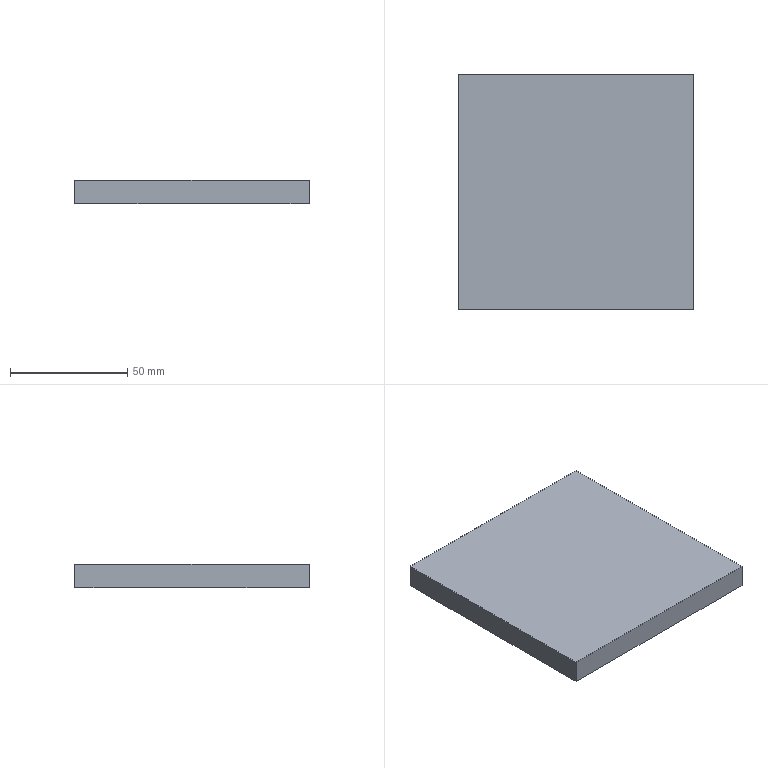Part | NX | features solid 2 | 1 solid | 13 faces | box 100 x 100 x 10 mm | volume 100000 mm3 | plane 13
STEP:
#1=CARTESIAN_POINT('',(490.,-590.,-30.));
#2=VERTEX_POINT('',#1);
#3=CARTESIAN_POINT('',(480.,-590.,-30.));
#4=VERTEX_POINT('',#3);
#5=CARTESIAN_POINT('',(490.,-590.,-30.));
#6=DIRECTION('',(-1.,0.,0.));
#7=VECTOR('',#6,1000.);
#8=LINE('',#5,#7);
#9=EDGE_CURVE('',#2,#4,#8,.T.);
#10=ORIENTED_EDGE('',*,*,#9,.T.);
#11=CARTESIAN_POINT('',(490.,-580.,-30.));
#12=VERTEX_POINT('',#11);
#13=CARTESIAN_POINT('',(430.,-640.,-30.));
#14=DIRECTION('',(0.7071,0.7071,0.));
#15=VECTOR('',#14,1000.);
#16=LINE('',#13,#15);
#17=EDGE_CURVE('',#4,#12,#16,.T.);
#18=ORIENTED_EDGE('',*,*,#17,.T.);
#19=CARTESIAN_POINT('',(490.,-490.,-30.));
#20=DIRECTION('',(0.,-1.,0.));
#21=VECTOR('',#20,1000.);
#22=LINE('',#19,#21);
#23=EDGE_CURVE('',#12,#2,#22,.T.);
#24=ORIENTED_EDGE('',*,*,#23,.T.);
#25=EDGE_LOOP('',(#10,#18,#24));
#26=FACE_BOUND('',#25,.T.);
#27=CARTESIAN_POINT('',(500.,-490.,-30.));
#28=DIRECTION('',(0.,0.,-1.));
#29=DIRECTION('',(0.,-1.,0.));
#30=AXIS2_PLACEMENT_3D('',#27,#28,#29);
#31=PLANE('',#30);
#32=ADVANCED_FACE('',(#26),#31,.T.);
#33=ORIENTED_EDGE('',*,*,#17,.F.);
#34=CARTESIAN_POINT('',(450.,-590.,-30.));
#35=VERTEX_POINT('',#34);
#36=CARTESIAN_POINT('',(490.,-590.,-30.));
#37=DIRECTION('',(-1.,0.,0.));
#38=VECTOR('',#37,1000.);
#39=LINE('',#36,#38);
#40=EDGE_CURVE('',#4,#35,#39,.T.);
#41=ORIENTED_EDGE('',*,*,#40,.T.);
#42=CARTESIAN_POINT('',(490.,-550.,-30.));
#43=VERTEX_POINT('',#42);
#44=CARTESIAN_POINT('',(400.,-640.,-30.));
#45=DIRECTION('',(0.7071,0.7071,0.));
#46=VECTOR('',#45,1000.);
#47=LINE('',#44,#46);
#48=EDGE_CURVE('',#35,#43,#47,.T.);
#49=ORIENTED_EDGE('',*,*,#48,.T.);
#50=CARTESIAN_POINT('',(490.,-490.,-30.));
#51=DIRECTION('',(0.,-1.,0.));
#52=VECTOR('',#51,1000.);
#53=LINE('',#50,#52);
#54=EDGE_CURVE('',#43,#12,#53,.T.);
#55=ORIENTED_EDGE('',*,*,#54,.T.);
#56=EDGE_LOOP('',(#33,#41,#49,#55));
#57=FACE_BOUND('',#56,.T.);
#58=CARTESIAN_POINT('',(500.,-490.,-30.));
#59=DIRECTION('',(0.,0.,-1.));
#60=DIRECTION('',(0.,-1.,0.));
#61=AXIS2_PLACEMENT_3D('',#58,#59,#60);
#62=PLANE('',#61);
#63=ADVANCED_FACE('',(#57),#62,.T.);
#64=ORIENTED_EDGE('',*,*,#48,.F.);
#65=CARTESIAN_POINT('',(420.,-590.,-30.));
#66=VERTEX_POINT('',#65);
#67=CARTESIAN_POINT('',(490.,-590.,-30.));
#68=DIRECTION('',(-1.,0.,0.));
#69=VECTOR('',#68,1000.);
#70=LINE('',#67,#69);
#71=EDGE_CURVE('',#35,#66,#70,.T.);
#72=ORIENTED_EDGE('',*,*,#71,.T.);
#73=CARTESIAN_POINT('',(490.,-520.,-30.));
#74=VERTEX_POINT('',#73);
#75=CARTESIAN_POINT('',(370.,-640.,-30.));
#76=DIRECTION('',(0.7071,0.7071,0.));
#77=VECTOR('',#76,1000.);
#78=LINE('',#75,#77);
#79=EDGE_CURVE('',#66,#74,#78,.T.);
#80=ORIENTED_EDGE('',*,*,#79,.T.);
#81=CARTESIAN_POINT('',(490.,-490.,-30.));
#82=DIRECTION('',(0.,-1.,0.));
#83=VECTOR('',#82,1000.);
#84=LINE('',#81,#83);
#85=EDGE_CURVE('',#74,#43,#84,.T.);
#86=ORIENTED_EDGE('',*,*,#85,.T.);
#87=EDGE_LOOP('',(#64,#72,#80,#86));
#88=FACE_BOUND('',#87,.T.);
#89=CARTESIAN_POINT('',(500.,-490.,-30.));
#90=DIRECTION('',(0.,0.,-1.));
#91=DIRECTION('',(0.,-1.,0.));
#92=AXIS2_PLACEMENT_3D('',#89,#90,#91);
#93=PLANE('',#92);
#94=ADVANCED_FACE('',(#88),#93,.T.);
#95=ORIENTED_EDGE('',*,*,#79,.F.);
#96=CARTESIAN_POINT('',(390.,-590.,-30.));
#97=VERTEX_POINT('',#96);
#98=CARTESIAN_POINT('',(490.,-590.,-30.));
#99=DIRECTION('',(-1.,0.,0.));
#100=VECTOR('',#99,1000.);
#101=LINE('',#98,#100);
#102=EDGE_CURVE('',#66,#97,#101,.T.);
#103=ORIENTED_EDGE('',*,*,#102,.T.);
#104=CARTESIAN_POINT('',(490.,-490.,-30.));
#105=VERTEX_POINT('',#104);
#106=CARTESIAN_POINT('',(340.,-640.,-30.));
#107=DIRECTION('',(0.7071,0.7071,0.));
#108=VECTOR('',#107,1000.);
#109=LINE('',#106,#108);
#110=EDGE_CURVE('',#97,#105,#109,.T.);
#111=ORIENTED_EDGE('',*,*,#110,.T.);
#112=CARTESIAN_POINT('',(490.,-490.,-30.));
#113=DIRECTION('',(0.,-1.,0.));
#114=VECTOR('',#113,1000.);
#115=LINE('',#112,#114);
#116=EDGE_CURVE('',#105,#74,#115,.T.);
#117=ORIENTED_EDGE('',*,*,#116,.T.);
#118=EDGE_LOOP('',(#95,#103,#111,#117));
#119=FACE_BOUND('',#118,.T.);
#120=CARTESIAN_POINT('',(500.,-490.,-30.));
#121=DIRECTION('',(0.,0.,-1.));
#122=DIRECTION('',(0.,-1.,0.));
#123=AXIS2_PLACEMENT_3D('',#120,#121,#122);
#124=PLANE('',#123);
#125=ADVANCED_FACE('',(#119),#124,.T.);
#126=CARTESIAN_POINT('',(390.,-560.,-30.));
#127=VERTEX_POINT('',#126);
#128=CARTESIAN_POINT('',(390.,-490.,-30.));
#129=DIRECTION('',(0.,-1.,0.));
#130=VECTOR('',#129,1000.);
#131=LINE('',#128,#130);
#132=EDGE_CURVE('',#97,#127,#131,.F.);
#133=ORIENTED_EDGE('',*,*,#132,.T.);
#134=CARTESIAN_POINT('',(460.,-490.,-30.));
#135=VERTEX_POINT('',#134);
#136=CARTESIAN_POINT('',(310.,-640.,-30.));
#137=DIRECTION('',(0.7071,0.7071,0.));
#138=VECTOR('',#137,1000.);
#139=LINE('',#136,#138);
#140=EDGE_CURVE('',#127,#135,#139,.T.);
#141=ORIENTED_EDGE('',*,*,#140,.T.);
#142=CARTESIAN_POINT('',(500.,-490.,-30.));
#143=DIRECTION('',(1.,0.,0.));
#144=VECTOR('',#143,1000.);
#145=LINE('',#142,#144);
#146=EDGE_CURVE('',#105,#135,#145,.F.);
#147=ORIENTED_EDGE('',*,*,#146,.F.);
#148=ORIENTED_EDGE('',*,*,#110,.F.);
#149=EDGE_LOOP('',(#133,#141,#147,#148));
#150=FACE_BOUND('',#149,.T.);
#151=CARTESIAN_POINT('',(500.,-490.,-30.));
#152=DIRECTION('',(0.,0.,-1.));
#153=DIRECTION('',(0.,-1.,0.));
#154=AXIS2_PLACEMENT_3D('',#151,#152,#153);
#155=PLANE('',#154);
#156=ADVANCED_FACE('',(#150),#155,.T.);
#157=CARTESIAN_POINT('',(390.,-530.,-30.));
#158=VERTEX_POINT('',#157);
#159=CARTESIAN_POINT('',(390.,-590.,-30.));
#160=DIRECTION('',(0.,1.,0.));
#161=VECTOR('',#160,1000.);
#162=LINE('',#159,#161);
#163=EDGE_CURVE('',#158,#127,#162,.F.);
#164=ORIENTED_EDGE('',*,*,#163,.F.);
#165=CARTESIAN_POINT('',(430.,-490.,-30.));
#166=VERTEX_POINT('',#165);
#167=CARTESIAN_POINT('',(280.,-640.,-30.));
#168=DIRECTION('',(0.7071,0.7071,0.));
#169=VECTOR('',#168,1000.);
#170=LINE('',#167,#169);
#171=EDGE_CURVE('',#158,#166,#170,.T.);
#172=ORIENTED_EDGE('',*,*,#171,.T.);
#173=CARTESIAN_POINT('',(500.,-490.,-30.));
#174=DIRECTION('',(1.,0.,0.));
#175=VECTOR('',#174,1000.);
#176=LINE('',#173,#175);
#177=EDGE_CURVE('',#135,#166,#176,.F.);
#178=ORIENTED_EDGE('',*,*,#177,.F.);
#179=ORIENTED_EDGE('',*,*,#140,.F.);
#180=EDGE_LOOP('',(#164,#172,#178,#179));
#181=FACE_BOUND('',#180,.T.);
#182=CARTESIAN_POINT('',(500.,-490.,-30.));
#183=DIRECTION('',(0.,0.,-1.));
#184=DIRECTION('',(0.,-1.,0.));
#185=AXIS2_PLACEMENT_3D('',#182,#183,#184);
#186=PLANE('',#185);
#187=ADVANCED_FACE('',(#181),#186,.T.);
#188=CARTESIAN_POINT('',(390.,-490.,-30.));
#189=VERTEX_POINT('',#188);
#190=CARTESIAN_POINT('',(390.,-500.,-30.));
#191=VERTEX_POINT('',#190);
#192=CARTESIAN_POINT('',(390.,-590.,-30.));
#193=DIRECTION('',(0.,1.,0.));
#194=VECTOR('',#193,1000.);
#195=LINE('',#192,#194);
#196=EDGE_CURVE('',#189,#191,#195,.F.);
#197=ORIENTED_EDGE('',*,*,#196,.F.);
#198=CARTESIAN_POINT('',(400.,-490.,-30.));
#199=VERTEX_POINT('',#198);
#200=CARTESIAN_POINT('',(500.,-490.,-30.));
#201=DIRECTION('',(1.,0.,0.));
#202=VECTOR('',#201,1000.);
#203=LINE('',#200,#202);
#204=EDGE_CURVE('',#199,#189,#203,.F.);
#205=ORIENTED_EDGE('',*,*,#204,.F.);
#206=CARTESIAN_POINT('',(250.,-640.,-30.));
#207=DIRECTION('',(0.7071,0.7071,0.));
#208=VECTOR('',#207,1000.);
#209=LINE('',#206,#208);
#210=EDGE_CURVE('',#191,#199,#209,.T.);
#211=ORIENTED_EDGE('',*,*,#210,.F.);
#212=EDGE_LOOP('',(#197,#205,#211));
#213=FACE_BOUND('',#212,.T.);
#214=CARTESIAN_POINT('',(500.,-490.,-30.));
#215=DIRECTION('',(0.,0.,-1.));
#216=DIRECTION('',(0.,-1.,0.));
#217=AXIS2_PLACEMENT_3D('',#214,#215,#216);
#218=PLANE('',#217);
#219=ADVANCED_FACE('',(#213),#218,.T.);
#220=ORIENTED_EDGE('',*,*,#171,.F.);
#221=CARTESIAN_POINT('',(390.,-590.,-30.));
#222=DIRECTION('',(0.,1.,0.));
#223=VECTOR('',#222,1000.);
#224=LINE('',#221,#223);
#225=EDGE_CURVE('',#191,#158,#224,.F.);
#226=ORIENTED_EDGE('',*,*,#225,.F.);
#227=ORIENTED_EDGE('',*,*,#210,.T.);
#228=CARTESIAN_POINT('',(500.,-490.,-30.));
#229=DIRECTION('',(1.,0.,0.));
#230=VECTOR('',#229,1000.);
#231=LINE('',#228,#230);
#232=EDGE_CURVE('',#166,#199,#231,.F.);
#233=ORIENTED_EDGE('',*,*,#232,.F.);
#234=EDGE_LOOP('',(#220,#226,#227,#233));
#235=FACE_BOUND('',#234,.T.);
#236=CARTESIAN_POINT('',(500.,-490.,-30.));
#237=DIRECTION('',(0.,0.,-1.));
#238=DIRECTION('',(0.,-1.,0.));
#239=AXIS2_PLACEMENT_3D('',#236,#237,#238);
#240=PLANE('',#239);
#241=ADVANCED_FACE('',(#235),#240,.T.);
#242=ORIENTED_EDGE('',*,*,#146,.T.);
#243=ORIENTED_EDGE('',*,*,#177,.T.);
#244=ORIENTED_EDGE('',*,*,#232,.T.);
#245=ORIENTED_EDGE('',*,*,#204,.T.);
#246=CARTESIAN_POINT('',(390.,-490.,-20.));
#247=VERTEX_POINT('',#246);
#248=CARTESIAN_POINT('',(390.,-490.,-30.));
#249=DIRECTION('',(0.,0.,1.));
#250=VECTOR('',#249,1000.);
#251=LINE('',#248,#250);
#252=EDGE_CURVE('',#189,#247,#251,.T.);
#253=ORIENTED_EDGE('',*,*,#252,.T.);
#254=CARTESIAN_POINT('',(490.,-490.,-20.));
#255=VERTEX_POINT('',#254);
#256=CARTESIAN_POINT('',(500.,-490.,-20.));
#257=DIRECTION('',(1.,0.,0.));
#258=VECTOR('',#257,1000.);
#259=LINE('',#256,#258);
#260=EDGE_CURVE('',#255,#247,#259,.F.);
#261=ORIENTED_EDGE('',*,*,#260,.F.);
#262=CARTESIAN_POINT('',(490.,-490.,-30.));
#263=DIRECTION('',(0.,0.,-1.));
#264=VECTOR('',#263,1000.);
#265=LINE('',#262,#264);
#266=EDGE_CURVE('',#105,#255,#265,.F.);
#267=ORIENTED_EDGE('',*,*,#266,.F.);
#268=EDGE_LOOP('',(#242,#243,#244,#245,#253,#261,#267));
#269=FACE_BOUND('',#268,.T.);
#270=CARTESIAN_POINT('',(500.,-490.,-30.));
#271=DIRECTION('',(0.,-1.,0.));
#272=DIRECTION('',(0.,0.,1.));
#273=AXIS2_PLACEMENT_3D('',#270,#271,#272);
#274=PLANE('',#273);
#275=ADVANCED_FACE('',(#269),#274,.F.);
#276=CARTESIAN_POINT('',(490.,-590.,-20.));
#277=VERTEX_POINT('',#276);
#278=CARTESIAN_POINT('',(490.,-590.,-30.));
#279=DIRECTION('',(0.,0.,-1.));
#280=VECTOR('',#279,1000.);
#281=LINE('',#278,#280);
#282=EDGE_CURVE('',#2,#277,#281,.F.);
#283=ORIENTED_EDGE('',*,*,#282,.T.);
#284=CARTESIAN_POINT('',(390.,-590.,-20.));
#285=VERTEX_POINT('',#284);
#286=CARTESIAN_POINT('',(490.,-590.,-20.));
#287=DIRECTION('',(-1.,0.,0.));
#288=VECTOR('',#287,1000.);
#289=LINE('',#286,#288);
#290=EDGE_CURVE('',#277,#285,#289,.T.);
#291=ORIENTED_EDGE('',*,*,#290,.T.);
#292=CARTESIAN_POINT('',(390.,-590.,-30.));
#293=DIRECTION('',(0.,0.,-1.));
#294=VECTOR('',#293,1000.);
#295=LINE('',#292,#294);
#296=EDGE_CURVE('',#97,#285,#295,.F.);
#297=ORIENTED_EDGE('',*,*,#296,.F.);
#298=ORIENTED_EDGE('',*,*,#102,.F.);
#299=ORIENTED_EDGE('',*,*,#71,.F.);
#300=ORIENTED_EDGE('',*,*,#40,.F.);
#301=ORIENTED_EDGE('',*,*,#9,.F.);
#302=EDGE_LOOP('',(#283,#291,#297,#298,#299,#300,#301));
#303=FACE_BOUND('',#302,.T.);
#304=CARTESIAN_POINT('',(490.,-590.,-30.));
#305=DIRECTION('',(0.,-1.,0.));
#306=DIRECTION('',(0.,0.,-1.));
#307=AXIS2_PLACEMENT_3D('',#304,#305,#306);
#308=PLANE('',#307);
#309=ADVANCED_FACE('',(#303),#308,.T.);
#310=CARTESIAN_POINT('',(390.,-590.,-20.));
#311=DIRECTION('',(0.,1.,0.));
#312=VECTOR('',#311,1000.);
#313=LINE('',#310,#312);
#314=EDGE_CURVE('',#247,#285,#313,.F.);
#315=ORIENTED_EDGE('',*,*,#314,.F.);
#316=ORIENTED_EDGE('',*,*,#252,.F.);
#317=ORIENTED_EDGE('',*,*,#196,.T.);
#318=ORIENTED_EDGE('',*,*,#225,.T.);
#319=ORIENTED_EDGE('',*,*,#163,.T.);
#320=ORIENTED_EDGE('',*,*,#132,.F.);
#321=ORIENTED_EDGE('',*,*,#296,.T.);
#322=EDGE_LOOP('',(#315,#316,#317,#318,#319,#320,#321));
#323=FACE_BOUND('',#322,.T.);
#324=CARTESIAN_POINT('',(390.,-590.,-30.));
#325=DIRECTION('',(-1.,0.,0.));
#326=DIRECTION('',(0.,0.,1.));
#327=AXIS2_PLACEMENT_3D('',#324,#325,#326);
#328=PLANE('',#327);
#329=ADVANCED_FACE('',(#323),#328,.T.);
#330=CARTESIAN_POINT('',(490.,-490.,-20.));
#331=DIRECTION('',(0.,-1.,0.));
#332=VECTOR('',#331,1000.);
#333=LINE('',#330,#332);
#334=EDGE_CURVE('',#255,#277,#333,.T.);
#335=ORIENTED_EDGE('',*,*,#334,.T.);
#336=ORIENTED_EDGE('',*,*,#282,.F.);
#337=ORIENTED_EDGE('',*,*,#23,.F.);
#338=ORIENTED_EDGE('',*,*,#54,.F.);
#339=ORIENTED_EDGE('',*,*,#85,.F.);
#340=ORIENTED_EDGE('',*,*,#116,.F.);
#341=ORIENTED_EDGE('',*,*,#266,.T.);
#342=EDGE_LOOP('',(#335,#336,#337,#338,#339,#340,#341));
#343=FACE_BOUND('',#342,.T.);
#344=CARTESIAN_POINT('',(490.,-490.,-30.));
#345=DIRECTION('',(-1.,0.,0.));
#346=DIRECTION('',(0.,0.,-1.));
#347=AXIS2_PLACEMENT_3D('',#344,#345,#346);
#348=PLANE('',#347);
#349=ADVANCED_FACE('',(#343),#348,.F.);
#350=ORIENTED_EDGE('',*,*,#260,.T.);
#351=ORIENTED_EDGE('',*,*,#314,.T.);
#352=ORIENTED_EDGE('',*,*,#290,.F.);
#353=ORIENTED_EDGE('',*,*,#334,.F.);
#354=EDGE_LOOP('',(#350,#351,#352,#353));
#355=FACE_BOUND('',#354,.T.);
#356=CARTESIAN_POINT('',(340.,-490.,-20.));
#357=DIRECTION('',(0.,0.,-1.));
#358=DIRECTION('',(0.,-1.,0.));
#359=AXIS2_PLACEMENT_3D('',#356,#357,#358);
#360=PLANE('',#359);
#361=ADVANCED_FACE('',(#355),#360,.F.);
#362=CLOSED_SHELL('',(#32,#63,#94,#125,#156,#187,#219,#241,#275,#309,#329,#349,#361));
#363=MANIFOLD_SOLID_BREP('',#362);
#364=(LENGTH_UNIT()NAMED_UNIT(*)SI_UNIT(.MILLI.,.METRE.));
#365=UNCERTAINTY_MEASURE_WITH_UNIT(LENGTH_MEASURE(0.0508),#364,'','');
#366=(NAMED_UNIT(*)PLANE_ANGLE_UNIT()SI_UNIT($,.RADIAN.));
#367=(NAMED_UNIT(*)SI_UNIT($,.STERADIAN.)SOLID_ANGLE_UNIT());
#368=(GEOMETRIC_REPRESENTATION_CONTEXT(3)GLOBAL_UNCERTAINTY_ASSIGNED_CONTEXT((#365))GLOBAL_UNIT_ASSIGNED_CONTEXT((#364,#366,#367))REPRESENTATION_CONTEXT('',''));
#369=ADVANCED_BREP_SHAPE_REPRESENTATION('',(#363),#368);